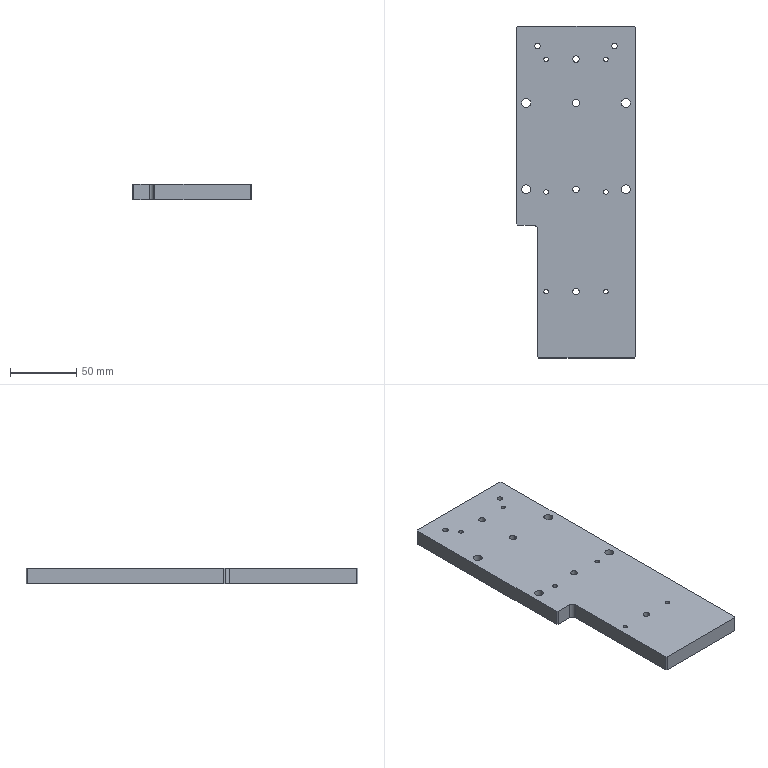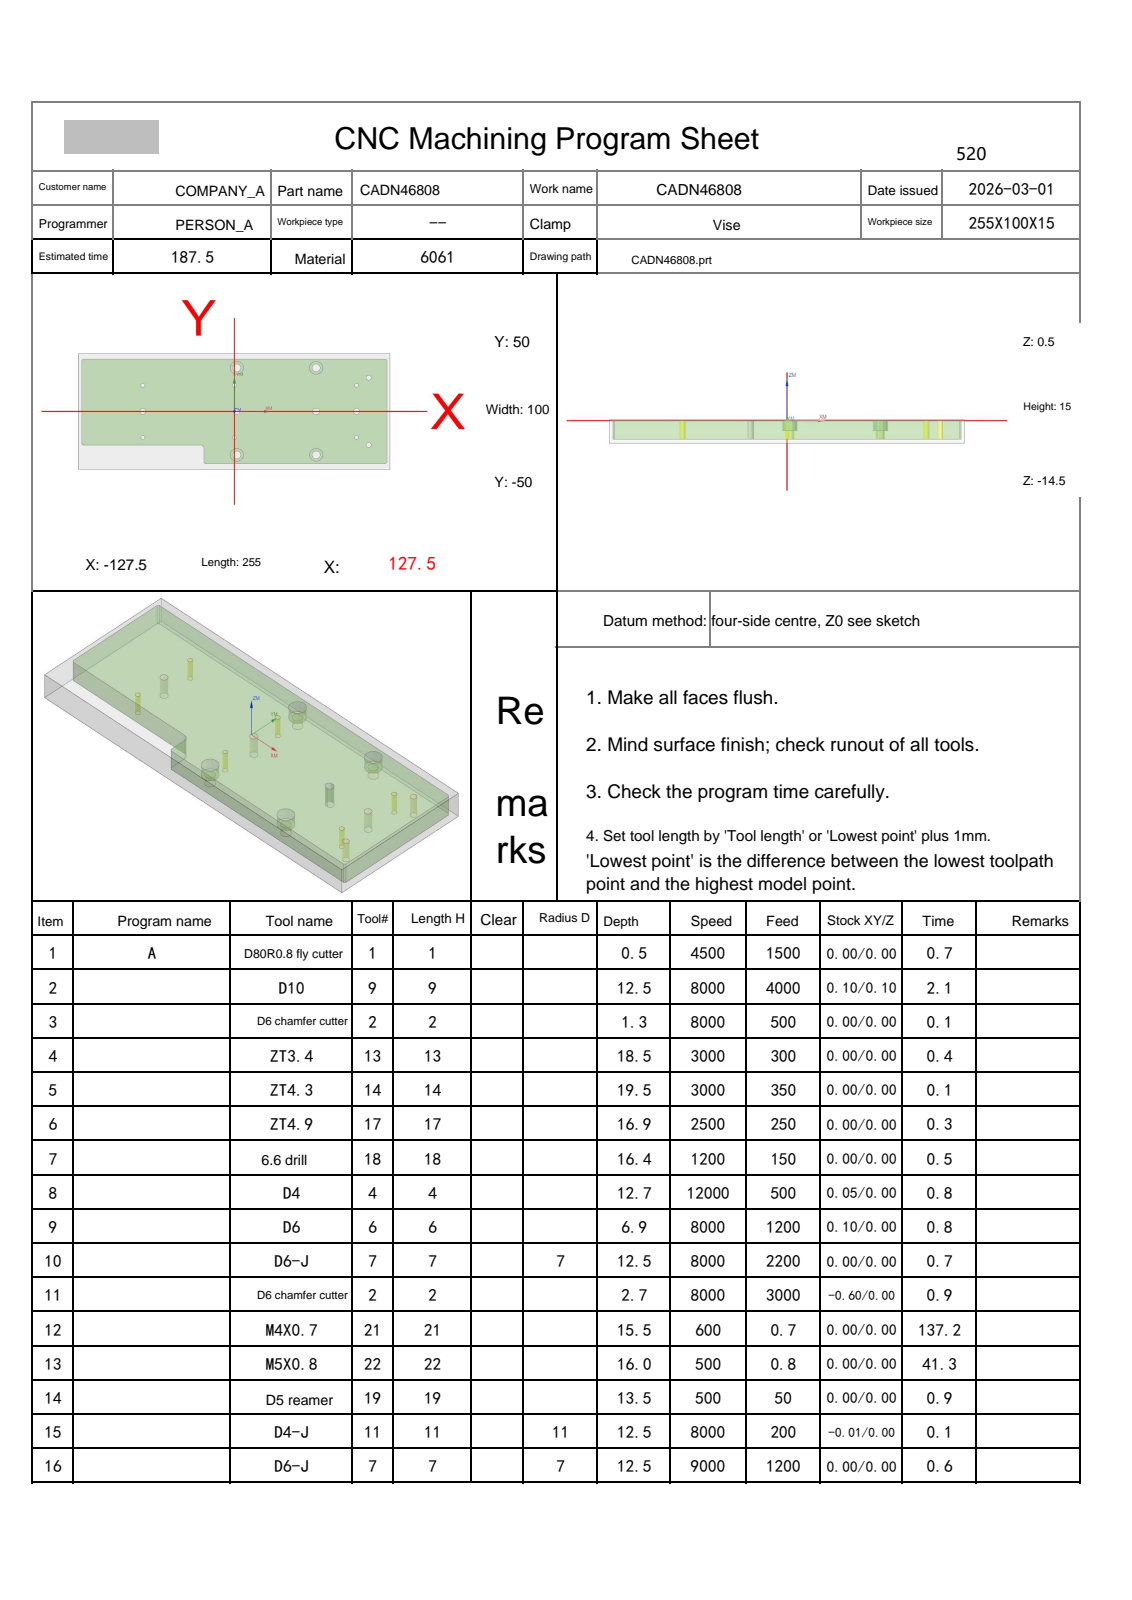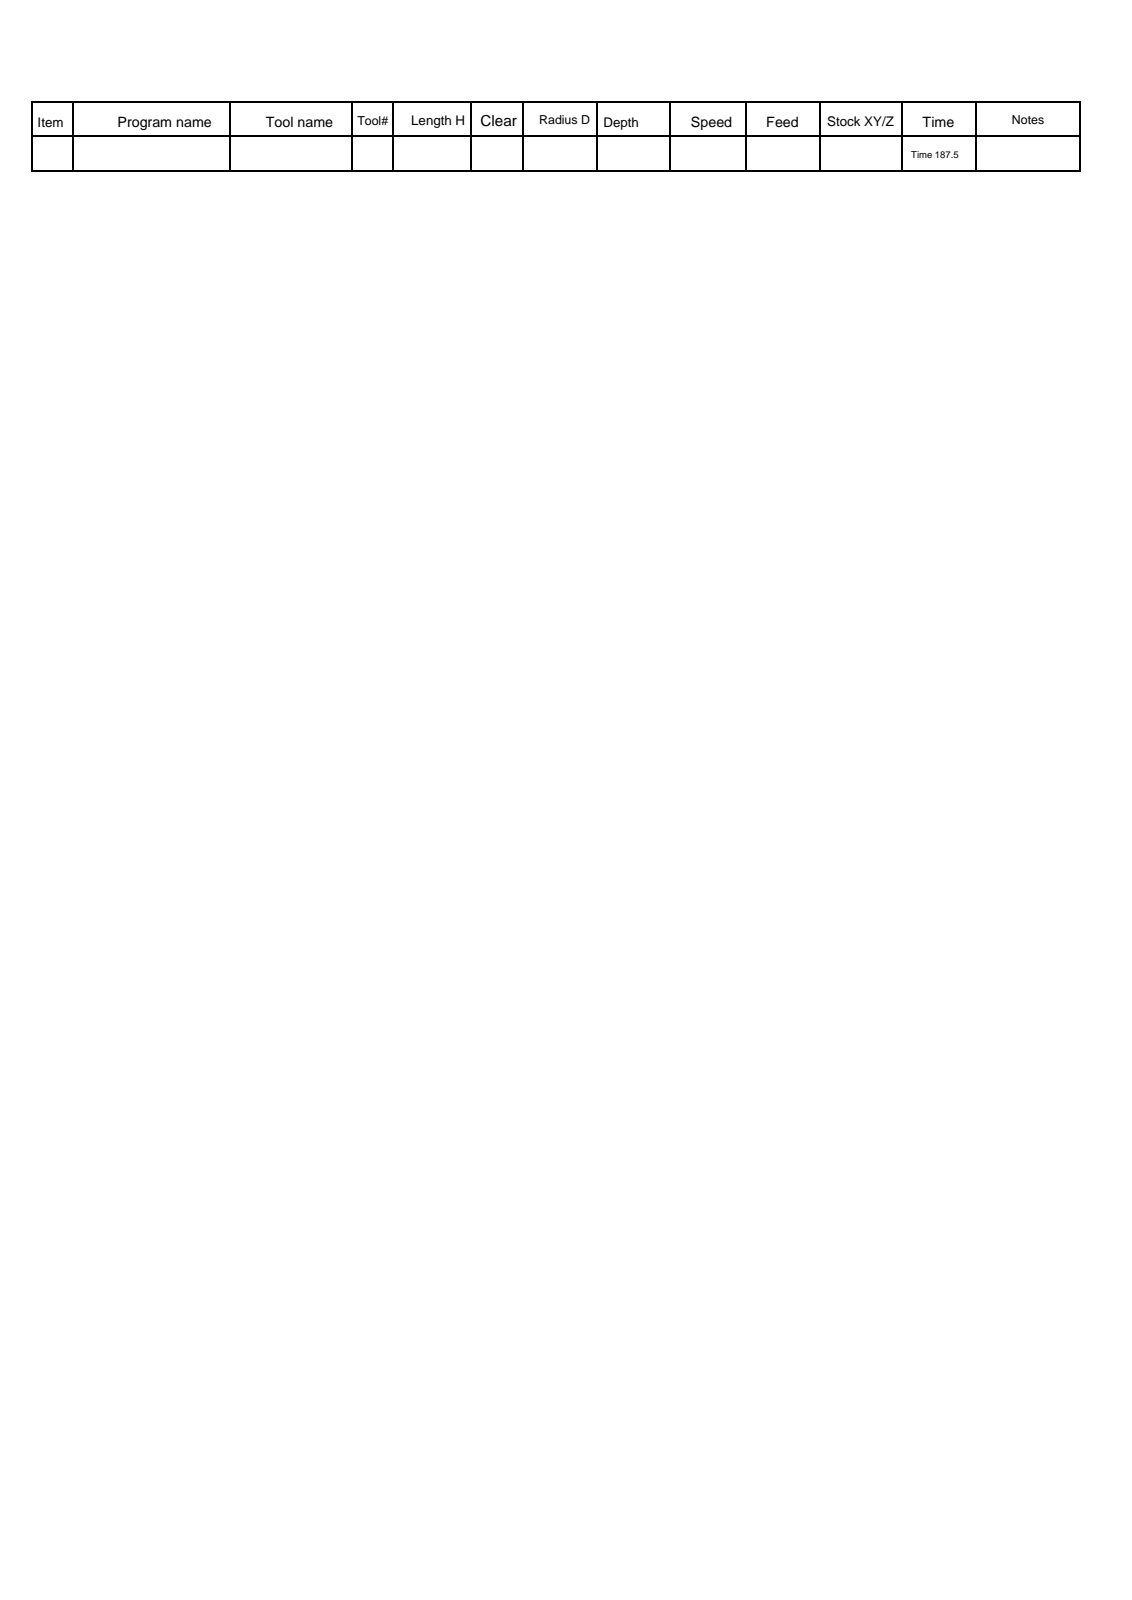NC program | NX | posted by the shop | part box 90 x 250 x 12 mm
Lines 1514 to 3445 of 3445, first 1356 of 1932 lines:
N10 T07 M06
(D6-J  D=6. R=0. H=07 ce=0.00 di=0.00)
G00 G90 G54 X2. Y-37.5 M03 S8000
G43 H07 Z50.
M08
Z0.0
G41 D07
G01 X2.197 Y-37.468 F500.
G03 X3.242 Y-36.242 I-.197 J1.226
X2. Y-35. I-1.242 J0.0
X2. Y-35. Z-5. I0.0 J-2.5
X-.456 Y-37.968 Z-6.4 I0.0 J-2.5
X2. Y-40. I2.456 J.468
X4.5 Y-37.5 I0.0 J2.5
X2. Y-35. I-2.5 J0.0
X-.5 Y-37.5 I0.0 J-2.5
X-.456 Y-37.968 I2.5 J0.0
X.764 Y-38.978 I1.22 J.233
X2.006 Y-37.736 I0.0 J1.242
G01 Y-37.7
G40 X2. Y-37.5
G00 Z50.
X67.
Z0.0
G41 D07
G01 X67.197 Y-37.468
G03 X68.242 Y-36.242 I-.197 J1.226
X67. Y-35. I-1.242 J0.0
X67. Y-35. Z-5. I0.0 J-2.5
X64.544 Y-37.968 Z-6.4 I0.0 J-2.5
X67. Y-40. I2.456 J.468
X69.5 Y-37.5 I0.0 J2.5
X67. Y-35. I-2.5 J0.0
X64.5 Y-37.5 I0.0 J-2.5
X64.544 Y-37.968 I2.5 J0.0
X65.764 Y-38.978 I1.22 J.233
X67.006 Y-37.736 I0.0 J1.242
G01 Y-37.7
G40 X67. Y-37.5
G00 Z50.
Y37.5
Z0.0
G41 D07
G01 X67.197 Y37.532
G03 X68.242 Y38.758 I-.197 J1.226
X67. Y40. I-1.242 J0.0
X67. Y40. Z-5. I0.0 J-2.5
X64.544 Y37.032 Z-6.4 I0.0 J-2.5
X67. Y35. I2.456 J.468
X69.5 Y37.5 I0.0 J2.5
X67. Y40. I-2.5 J0.0
X64.5 Y37.5 I0.0 J-2.5
X64.544 Y37.032 I2.5 J0.0
X65.764 Y36.022 I1.22 J.233
X67.006 Y37.264 I0.0 J1.242
G01 Y37.3
G40 X67. Y37.5
G00 Z50.
X2.
Z0.0
G41 D07
G01 X2.197 Y37.532
G03 X3.242 Y38.758 I-.197 J1.226
X2. Y40. I-1.242 J0.0
X2. Y40. Z-5. I0.0 J-2.5
X-.456 Y37.032 Z-6.4 I0.0 J-2.5
X2. Y35. I2.456 J.468
X4.5 Y37.5 I0.0 J2.5
X2. Y40. I-2.5 J0.0
X-.5 Y37.5 I0.0 J-2.5
X-.456 Y37.032 I2.5 J0.0
X.764 Y36.022 I1.22 J.233
X2.006 Y37.264 I0.0 J1.242
G01 Y37.3
G40 X2. Y37.5
G00 Z50.
G00 G90 X-28.61 Y-35.604 M03 S8000
Z50.
Z.35
G01 X-28.602 Y-35.602 Z.259 F2200.
X-28.581 Y-35.597 Z.177
X-28.547 Y-35.587 Z.103
X-28.503 Y-35.573 Z.038
X-28.452 Y-35.555 Z-.019
X-28.395 Y-35.531 Z-.069
X-28.336 Y-35.501 Z-.111
X-28.275 Y-35.465 Z-.147
X-28.215 Y-35.422 Z-.177
X-28.158 Y-35.372 Z-.201
X-28.107 Y-35.315 Z-.22
X-28.063 Y-35.25 Z-.234
X-28.03 Y-35.176 Z-.243
X-28.008 Y-35.094 Z-.248
X-28. Y-35.003 Z-.25
Y-32.
X-31.003
X-31.072 Y-32.016 Z-.251
X-31.117 Y-32.062 Z-.253
X-31.139 Y-32.135 Z-.256
X-31.141 Y-32.231 Z-.261
X-31.124 Y-32.347 Z-.267
X-31.089 Y-32.479 Z-.274
X-31.039 Y-32.624 Z-.281
X-30.975 Y-32.778 Z-.29
X-30.899 Y-32.939 Z-.298
X-30.812 Y-33.102 Z-.308
X-30.717 Y-33.264 Z-.318
X-30.484 Y-33.605 Z-.34
X-30.221 Y-33.924 Z-.363
X-29.929 Y-34.217 Z-.387
X-29.61 Y-34.481 Z-.41
X-29.268 Y-34.715 Z-.432
X-29.106 Y-34.81 Z-.442
X-28.943 Y-34.897 Z-.452
X-28.782 Y-34.973 Z-.46
X-28.627 Y-35.038 Z-.469
X-28.481 Y-35.088 Z-.476
X-28.349 Y-35.123 Z-.483
X-28.232 Y-35.141 Z-.489
X-28.136 Y-35.139 Z-.494
X-28.063 Y-35.117 Z-.497
X-28.016 Y-35.072 Z-.499
X-28. Y-35.003 Z-.5
Y-32.
X-31.003
X-31.072 Y-32.016 Z-.501
X-31.117 Y-32.062 Z-.503
X-31.139 Y-32.135 Z-.506
X-31.141 Y-32.231 Z-.511
X-31.124 Y-32.347 Z-.517
X-31.089 Y-32.479 Z-.524
X-31.039 Y-32.624 Z-.531
X-30.975 Y-32.778 Z-.54
X-30.899 Y-32.939 Z-.548
X-30.812 Y-33.102 Z-.558
X-30.717 Y-33.264 Z-.568
X-30.484 Y-33.605 Z-.59
X-30.221 Y-33.924 Z-.613
X-29.929 Y-34.217 Z-.637
X-29.61 Y-34.481 Z-.66
X-29.268 Y-34.715 Z-.682
X-29.106 Y-34.81 Z-.692
X-28.943 Y-34.897 Z-.702
X-28.782 Y-34.973 Z-.71
X-28.627 Y-35.038 Z-.719
X-28.481 Y-35.088 Z-.726
X-28.349 Y-35.123 Z-.733
X-28.232 Y-35.141 Z-.739
X-28.136 Y-35.139 Z-.744
X-28.063 Y-35.117 Z-.747
X-28.016 Y-35.072 Z-.749
X-28. Y-35.003 Z-.75
Y-32.
X-31.003
X-31.072 Y-32.016 Z-.751
X-31.117 Y-32.062 Z-.753
X-31.139 Y-32.135 Z-.756
X-31.141 Y-32.231 Z-.761
X-31.124 Y-32.347 Z-.767
X-31.089 Y-32.479 Z-.774
X-31.039 Y-32.624 Z-.781
X-30.975 Y-32.778 Z-.79
X-30.899 Y-32.939 Z-.798
X-30.812 Y-33.102 Z-.808
X-30.717 Y-33.264 Z-.818
X-30.484 Y-33.605 Z-.84
X-30.221 Y-33.924 Z-.863
X-29.929 Y-34.217 Z-.887
X-29.61 Y-34.481 Z-.91
X-29.268 Y-34.715 Z-.932
X-29.106 Y-34.81 Z-.942
X-28.943 Y-34.897 Z-.952
X-28.782 Y-34.973 Z-.96
X-28.627 Y-35.038 Z-.969
X-28.481 Y-35.088 Z-.976
X-28.349 Y-35.123 Z-.983
X-28.232 Y-35.141 Z-.989
X-28.136 Y-35.139 Z-.994
X-28.063 Y-35.117 Z-.997
X-28.016 Y-35.072 Z-.999
X-28. Y-35.003 Z-1.
Y-32.
X-31.003
X-31.072 Y-32.016 Z-1.001
X-31.117 Y-32.062 Z-1.003
X-31.139 Y-32.135 Z-1.006
X-31.141 Y-32.231 Z-1.011
X-31.124 Y-32.347 Z-1.017
X-31.089 Y-32.479 Z-1.024
X-31.039 Y-32.624 Z-1.031
X-30.975 Y-32.778 Z-1.04
X-30.899 Y-32.939 Z-1.048
X-30.812 Y-33.102 Z-1.058
X-30.717 Y-33.264 Z-1.068
X-30.484 Y-33.605 Z-1.09
X-30.221 Y-33.924 Z-1.113
X-29.929 Y-34.217 Z-1.137
X-29.61 Y-34.481 Z-1.16
X-29.268 Y-34.715 Z-1.182
X-29.106 Y-34.81 Z-1.192
X-28.943 Y-34.897 Z-1.202
X-28.782 Y-34.973 Z-1.21
X-28.627 Y-35.038 Z-1.219
X-28.481 Y-35.088 Z-1.226
X-28.349 Y-35.123 Z-1.233
X-28.232 Y-35.141 Z-1.239
X-28.136 Y-35.139 Z-1.244
X-28.063 Y-35.117 Z-1.247
X-28.016 Y-35.072 Z-1.249
X-28. Y-35.003 Z-1.25
Y-32.
X-31.003
X-31.072 Y-32.016 Z-1.251
X-31.117 Y-32.062 Z-1.253
X-31.139 Y-32.135 Z-1.256
X-31.141 Y-32.231 Z-1.261
X-31.124 Y-32.347 Z-1.267
X-31.089 Y-32.479 Z-1.274
X-31.039 Y-32.624 Z-1.281
X-30.975 Y-32.778 Z-1.29
X-30.899 Y-32.939 Z-1.298
X-30.812 Y-33.102 Z-1.308
X-30.717 Y-33.264 Z-1.318
X-30.484 Y-33.605 Z-1.34
X-30.221 Y-33.924 Z-1.363
X-29.929 Y-34.217 Z-1.387
X-29.61 Y-34.481 Z-1.41
X-29.268 Y-34.715 Z-1.432
X-29.106 Y-34.81 Z-1.442
X-28.943 Y-34.897 Z-1.452
X-28.782 Y-34.973 Z-1.46
X-28.627 Y-35.038 Z-1.469
X-28.481 Y-35.088 Z-1.476
X-28.349 Y-35.123 Z-1.483
X-28.232 Y-35.141 Z-1.489
X-28.136 Y-35.139 Z-1.494
X-28.063 Y-35.117 Z-1.497
X-28.016 Y-35.072 Z-1.499
X-28. Y-35.003 Z-1.5
Y-32.
X-31.003
X-31.072 Y-32.016 Z-1.501
X-31.117 Y-32.062 Z-1.503
X-31.139 Y-32.135 Z-1.506
X-31.141 Y-32.231 Z-1.511
X-31.124 Y-32.347 Z-1.517
X-31.089 Y-32.479 Z-1.524
X-31.039 Y-32.624 Z-1.531
X-30.975 Y-32.778 Z-1.54
X-30.899 Y-32.939 Z-1.548
X-30.812 Y-33.102 Z-1.558
X-30.717 Y-33.264 Z-1.568
X-30.484 Y-33.605 Z-1.59
X-30.221 Y-33.924 Z-1.613
X-29.929 Y-34.217 Z-1.637
X-29.61 Y-34.481 Z-1.66
X-29.268 Y-34.715 Z-1.682
X-29.106 Y-34.81 Z-1.692
X-28.943 Y-34.897 Z-1.702
X-28.782 Y-34.973 Z-1.71
X-28.627 Y-35.038 Z-1.719
X-28.481 Y-35.088 Z-1.726
X-28.349 Y-35.123 Z-1.733
X-28.232 Y-35.141 Z-1.739
X-28.136 Y-35.139 Z-1.744
X-28.063 Y-35.117 Z-1.747
X-28.016 Y-35.072 Z-1.749
X-28. Y-35.003 Z-1.75
Y-32.
X-31.003
X-31.072 Y-32.016 Z-1.751
X-31.117 Y-32.062 Z-1.753
X-31.139 Y-32.135 Z-1.756
X-31.141 Y-32.231 Z-1.761
X-31.124 Y-32.347 Z-1.767
X-31.089 Y-32.479 Z-1.774
X-31.039 Y-32.624 Z-1.781
X-30.975 Y-32.778 Z-1.79
X-30.899 Y-32.939 Z-1.798
X-30.812 Y-33.102 Z-1.808
X-30.717 Y-33.264 Z-1.818
X-30.484 Y-33.605 Z-1.84
X-30.221 Y-33.924 Z-1.863
X-29.929 Y-34.217 Z-1.887
X-29.61 Y-34.481 Z-1.91
X-29.268 Y-34.715 Z-1.932
X-29.106 Y-34.81 Z-1.942
X-28.943 Y-34.897 Z-1.952
X-28.782 Y-34.973 Z-1.96
X-28.627 Y-35.038 Z-1.969
X-28.481 Y-35.088 Z-1.976
X-28.349 Y-35.123 Z-1.983
X-28.232 Y-35.141 Z-1.989
X-28.136 Y-35.139 Z-1.994
X-28.063 Y-35.117 Z-1.997
X-28.016 Y-35.072 Z-1.999
X-28. Y-35.003 Z-2.
Y-32.
X-31.003
X-31.072 Y-32.016 Z-2.001
X-31.117 Y-32.062 Z-2.003
X-31.139 Y-32.135 Z-2.006
X-31.141 Y-32.231 Z-2.011
X-31.124 Y-32.347 Z-2.017
X-31.089 Y-32.479 Z-2.024
X-31.039 Y-32.624 Z-2.031
X-30.975 Y-32.778 Z-2.04
X-30.899 Y-32.939 Z-2.048
X-30.812 Y-33.102 Z-2.058
X-30.717 Y-33.264 Z-2.068
X-30.484 Y-33.605 Z-2.09
X-30.221 Y-33.924 Z-2.113
X-29.929 Y-34.217 Z-2.137
X-29.61 Y-34.481 Z-2.16
X-29.268 Y-34.715 Z-2.182
X-29.106 Y-34.81 Z-2.192
X-28.943 Y-34.897 Z-2.202
X-28.782 Y-34.973 Z-2.21
X-28.627 Y-35.038 Z-2.219
X-28.481 Y-35.088 Z-2.226
X-28.349 Y-35.123 Z-2.233
X-28.232 Y-35.141 Z-2.239
X-28.136 Y-35.139 Z-2.244
X-28.063 Y-35.117 Z-2.247
X-28.016 Y-35.072 Z-2.249
X-28. Y-35.003 Z-2.25
Y-32.
X-31.003
X-31.072 Y-32.016 Z-2.251
X-31.117 Y-32.062 Z-2.253
X-31.139 Y-32.135 Z-2.256
X-31.141 Y-32.231 Z-2.261
X-31.124 Y-32.347 Z-2.267
X-31.089 Y-32.479 Z-2.274
X-31.039 Y-32.624 Z-2.281
X-30.975 Y-32.778 Z-2.29
X-30.899 Y-32.939 Z-2.298
X-30.812 Y-33.102 Z-2.308
X-30.717 Y-33.264 Z-2.318
X-30.484 Y-33.605 Z-2.34
X-30.221 Y-33.924 Z-2.363
X-29.929 Y-34.217 Z-2.387
X-29.61 Y-34.481 Z-2.41
X-29.268 Y-34.715 Z-2.432
X-29.106 Y-34.81 Z-2.442
X-28.943 Y-34.897 Z-2.452
X-28.782 Y-34.973 Z-2.46
X-28.627 Y-35.038 Z-2.469
X-28.481 Y-35.088 Z-2.476
X-28.349 Y-35.123 Z-2.483
X-28.232 Y-35.141 Z-2.489
X-28.136 Y-35.139 Z-2.494
X-28.063 Y-35.117 Z-2.497
X-28.016 Y-35.072 Z-2.499
X-28. Y-35.003 Z-2.5
Y-32.
X-31.003
X-31.072 Y-32.016 Z-2.501
X-31.117 Y-32.062 Z-2.503
X-31.139 Y-32.135 Z-2.506
X-31.141 Y-32.231 Z-2.511
X-31.124 Y-32.347 Z-2.517
X-31.089 Y-32.479 Z-2.524
X-31.039 Y-32.624 Z-2.531
X-30.975 Y-32.778 Z-2.54
X-30.899 Y-32.939 Z-2.548
X-30.812 Y-33.102 Z-2.558
X-30.717 Y-33.264 Z-2.568
X-30.484 Y-33.605 Z-2.59
X-30.221 Y-33.924 Z-2.613
X-29.929 Y-34.217 Z-2.637
X-29.61 Y-34.481 Z-2.66
X-29.268 Y-34.715 Z-2.682
X-29.106 Y-34.81 Z-2.692
X-28.943 Y-34.897 Z-2.702
X-28.782 Y-34.973 Z-2.71
X-28.627 Y-35.038 Z-2.719
X-28.481 Y-35.088 Z-2.726
X-28.349 Y-35.123 Z-2.733
X-28.232 Y-35.141 Z-2.739
X-28.136 Y-35.139 Z-2.744
X-28.063 Y-35.117 Z-2.747
X-28.016 Y-35.072 Z-2.749
X-28. Y-35.003 Z-2.75
Y-32.
X-31.003
X-31.072 Y-32.016 Z-2.751
X-31.117 Y-32.062 Z-2.753
X-31.139 Y-32.135 Z-2.756
X-31.141 Y-32.231 Z-2.761
X-31.124 Y-32.347 Z-2.767
X-31.089 Y-32.479 Z-2.774
X-31.039 Y-32.624 Z-2.781
X-30.975 Y-32.778 Z-2.79
X-30.899 Y-32.939 Z-2.798
X-30.812 Y-33.102 Z-2.808
X-30.717 Y-33.264 Z-2.818
X-30.484 Y-33.605 Z-2.84
X-30.221 Y-33.924 Z-2.863
X-29.929 Y-34.217 Z-2.887
X-29.61 Y-34.481 Z-2.91
X-29.268 Y-34.715 Z-2.932
X-29.106 Y-34.81 Z-2.942
X-28.943 Y-34.897 Z-2.952
X-28.782 Y-34.973 Z-2.96
X-28.627 Y-35.038 Z-2.969
X-28.481 Y-35.088 Z-2.976
X-28.349 Y-35.123 Z-2.983
X-28.232 Y-35.141 Z-2.989
X-28.136 Y-35.139 Z-2.994
X-28.063 Y-35.117 Z-2.997
X-28.016 Y-35.072 Z-2.999
X-28. Y-35.003 Z-3.
Y-32.
X-31.003
X-31.072 Y-32.016 Z-3.001
X-31.117 Y-32.062 Z-3.003
X-31.139 Y-32.135 Z-3.006
X-31.141 Y-32.231 Z-3.011
X-31.124 Y-32.347 Z-3.017
X-31.089 Y-32.479 Z-3.024
X-31.039 Y-32.624 Z-3.031
X-30.975 Y-32.778 Z-3.04
X-30.899 Y-32.939 Z-3.048
X-30.812 Y-33.102 Z-3.058
X-30.717 Y-33.264 Z-3.068
X-30.484 Y-33.605 Z-3.09
X-30.221 Y-33.924 Z-3.113
X-29.929 Y-34.217 Z-3.137
X-29.61 Y-34.481 Z-3.16
X-29.268 Y-34.715 Z-3.182
X-29.106 Y-34.81 Z-3.192
X-28.943 Y-34.897 Z-3.202
X-28.782 Y-34.973 Z-3.21
X-28.627 Y-35.038 Z-3.219
X-28.481 Y-35.088 Z-3.226
X-28.349 Y-35.123 Z-3.233
X-28.232 Y-35.141 Z-3.239
X-28.136 Y-35.139 Z-3.244
X-28.063 Y-35.117 Z-3.247
X-28.016 Y-35.072 Z-3.249
X-28. Y-35.003 Z-3.25
Y-32.
X-31.003
X-31.072 Y-32.016 Z-3.251
X-31.117 Y-32.062 Z-3.253
X-31.139 Y-32.135 Z-3.256
X-31.141 Y-32.231 Z-3.261
X-31.124 Y-32.347 Z-3.267
X-31.089 Y-32.479 Z-3.274
X-31.039 Y-32.624 Z-3.281
X-30.975 Y-32.778 Z-3.29
X-30.899 Y-32.939 Z-3.298
X-30.812 Y-33.102 Z-3.308
X-30.717 Y-33.264 Z-3.318
X-30.484 Y-33.605 Z-3.34
X-30.221 Y-33.924 Z-3.363
X-29.929 Y-34.217 Z-3.387
X-29.61 Y-34.481 Z-3.41
X-29.268 Y-34.715 Z-3.432
X-29.106 Y-34.81 Z-3.442
X-28.943 Y-34.897 Z-3.452
X-28.782 Y-34.973 Z-3.46
X-28.627 Y-35.038 Z-3.469
X-28.481 Y-35.088 Z-3.476
X-28.349 Y-35.123 Z-3.483
X-28.232 Y-35.141 Z-3.489
X-28.136 Y-35.139 Z-3.494
X-28.063 Y-35.117 Z-3.497
X-28.016 Y-35.072 Z-3.499
X-28. Y-35.003 Z-3.5
Y-32.
X-31.003
X-31.072 Y-32.016 Z-3.501
X-31.117 Y-32.062 Z-3.503
X-31.139 Y-32.135 Z-3.506
X-31.141 Y-32.231 Z-3.511
X-31.124 Y-32.347 Z-3.517
X-31.089 Y-32.479 Z-3.524
X-31.039 Y-32.624 Z-3.531
X-30.975 Y-32.778 Z-3.54
X-30.899 Y-32.939 Z-3.548
X-30.812 Y-33.102 Z-3.558
X-30.717 Y-33.264 Z-3.568
X-30.484 Y-33.605 Z-3.59
X-30.221 Y-33.924 Z-3.613
X-29.929 Y-34.217 Z-3.637
X-29.61 Y-34.481 Z-3.66
X-29.268 Y-34.715 Z-3.682
X-29.106 Y-34.81 Z-3.692
X-28.943 Y-34.897 Z-3.702
X-28.782 Y-34.973 Z-3.71
X-28.627 Y-35.038 Z-3.719
X-28.481 Y-35.088 Z-3.726
X-28.349 Y-35.123 Z-3.733
X-28.232 Y-35.141 Z-3.739
X-28.136 Y-35.139 Z-3.744
X-28.063 Y-35.117 Z-3.747
X-28.016 Y-35.072 Z-3.749
X-28. Y-35.003 Z-3.75
Y-32.
X-31.003
X-31.072 Y-32.016 Z-3.751
X-31.117 Y-32.062 Z-3.753
X-31.139 Y-32.135 Z-3.756
X-31.141 Y-32.231 Z-3.761
X-31.124 Y-32.347 Z-3.767
X-31.089 Y-32.479 Z-3.774
X-31.039 Y-32.624 Z-3.781
X-30.975 Y-32.778 Z-3.79
X-30.899 Y-32.939 Z-3.798
X-30.812 Y-33.102 Z-3.808
X-30.717 Y-33.264 Z-3.818
X-30.484 Y-33.605 Z-3.84
X-30.221 Y-33.924 Z-3.863
X-29.929 Y-34.217 Z-3.887
X-29.61 Y-34.481 Z-3.91
X-29.268 Y-34.715 Z-3.932
X-29.106 Y-34.81 Z-3.942
X-28.943 Y-34.897 Z-3.952
X-28.782 Y-34.973 Z-3.96
X-28.627 Y-35.038 Z-3.969
X-28.481 Y-35.088 Z-3.976
X-28.349 Y-35.123 Z-3.983
X-28.232 Y-35.141 Z-3.989
X-28.136 Y-35.139 Z-3.994
X-28.063 Y-35.117 Z-3.997
X-28.016 Y-35.072 Z-3.999
X-28. Y-35.003 Z-4.
Y-32.
X-31.003
X-31.072 Y-32.016 Z-4.001
X-31.117 Y-32.062 Z-4.003
X-31.139 Y-32.135 Z-4.006
X-31.141 Y-32.231 Z-4.011
X-31.124 Y-32.347 Z-4.017
X-31.089 Y-32.479 Z-4.024
X-31.039 Y-32.624 Z-4.031
X-30.975 Y-32.778 Z-4.04
X-30.899 Y-32.939 Z-4.048
X-30.812 Y-33.102 Z-4.058
X-30.717 Y-33.264 Z-4.068
X-30.484 Y-33.605 Z-4.09
X-30.221 Y-33.924 Z-4.113
X-29.929 Y-34.217 Z-4.137
X-29.61 Y-34.481 Z-4.16
X-29.268 Y-34.715 Z-4.182
X-29.106 Y-34.81 Z-4.192
X-28.943 Y-34.897 Z-4.202
X-28.782 Y-34.973 Z-4.21
X-28.627 Y-35.038 Z-4.219
X-28.481 Y-35.088 Z-4.226
X-28.349 Y-35.123 Z-4.233
X-28.232 Y-35.141 Z-4.239
X-28.136 Y-35.139 Z-4.244
X-28.063 Y-35.117 Z-4.247
X-28.016 Y-35.072 Z-4.249
X-28. Y-35.003 Z-4.25
Y-32.
X-31.003
X-31.072 Y-32.016 Z-4.251
X-31.117 Y-32.062 Z-4.253
X-31.139 Y-32.135 Z-4.256
X-31.141 Y-32.231 Z-4.261
X-31.124 Y-32.347 Z-4.267
X-31.089 Y-32.479 Z-4.274
X-31.039 Y-32.624 Z-4.281
X-30.975 Y-32.778 Z-4.29
X-30.899 Y-32.939 Z-4.298
X-30.812 Y-33.102 Z-4.308
X-30.717 Y-33.264 Z-4.318
X-30.484 Y-33.605 Z-4.34
X-30.221 Y-33.924 Z-4.363
X-29.929 Y-34.217 Z-4.387
X-29.61 Y-34.481 Z-4.41
X-29.268 Y-34.715 Z-4.432
X-29.106 Y-34.81 Z-4.442
X-28.943 Y-34.897 Z-4.452
X-28.782 Y-34.973 Z-4.46
X-28.627 Y-35.038 Z-4.469
X-28.481 Y-35.088 Z-4.476
X-28.349 Y-35.123 Z-4.483
X-28.232 Y-35.141 Z-4.489
X-28.136 Y-35.139 Z-4.494
X-28.063 Y-35.117 Z-4.497
X-28.016 Y-35.072 Z-4.499
X-28. Y-35.003 Z-4.5
Y-32.
X-31.003
X-31.072 Y-32.016 Z-4.501
X-31.117 Y-32.062 Z-4.503
X-31.139 Y-32.135 Z-4.506
X-31.141 Y-32.231 Z-4.511
X-31.124 Y-32.347 Z-4.517
X-31.089 Y-32.479 Z-4.524
X-31.039 Y-32.624 Z-4.531
X-30.975 Y-32.778 Z-4.54
X-30.899 Y-32.939 Z-4.548
X-30.812 Y-33.102 Z-4.558
X-30.717 Y-33.264 Z-4.568
X-30.484 Y-33.605 Z-4.59
X-30.221 Y-33.924 Z-4.613
X-29.929 Y-34.217 Z-4.637
X-29.61 Y-34.481 Z-4.66
X-29.268 Y-34.715 Z-4.682
X-29.106 Y-34.81 Z-4.692
X-28.943 Y-34.897 Z-4.702
X-28.782 Y-34.973 Z-4.71
X-28.627 Y-35.038 Z-4.719
X-28.481 Y-35.088 Z-4.726
X-28.349 Y-35.123 Z-4.733
X-28.232 Y-35.141 Z-4.739
X-28.136 Y-35.139 Z-4.744
X-28.063 Y-35.117 Z-4.747
X-28.016 Y-35.072 Z-4.749
X-28. Y-35.003 Z-4.75
Y-32.
X-31.003
X-31.072 Y-32.016 Z-4.751
X-31.117 Y-32.062 Z-4.753
X-31.139 Y-32.135 Z-4.756
X-31.141 Y-32.231 Z-4.761
X-31.124 Y-32.347 Z-4.767
X-31.089 Y-32.479 Z-4.774
X-31.039 Y-32.624 Z-4.781
X-30.975 Y-32.778 Z-4.79
X-30.899 Y-32.939 Z-4.798
X-30.812 Y-33.102 Z-4.808
X-30.717 Y-33.264 Z-4.818
X-30.484 Y-33.605 Z-4.84
X-30.221 Y-33.924 Z-4.863
X-29.929 Y-34.217 Z-4.887
X-29.61 Y-34.481 Z-4.91
X-29.268 Y-34.715 Z-4.932
X-29.106 Y-34.81 Z-4.942
X-28.943 Y-34.897 Z-4.952
X-28.782 Y-34.973 Z-4.96
X-28.627 Y-35.038 Z-4.969
X-28.481 Y-35.088 Z-4.976
X-28.349 Y-35.123 Z-4.983
X-28.232 Y-35.141 Z-4.989
X-28.136 Y-35.139 Z-4.994
X-28.063 Y-35.117 Z-4.997
X-28.016 Y-35.072 Z-4.999
X-28. Y-35.003 Z-5.
Y-32.
X-31.003
X-31.072 Y-32.016 Z-5.001
X-31.117 Y-32.062 Z-5.003
X-31.139 Y-32.135 Z-5.006
X-31.141 Y-32.231 Z-5.011
X-31.124 Y-32.347 Z-5.017
X-31.089 Y-32.479 Z-5.024
X-31.039 Y-32.624 Z-5.031
X-30.975 Y-32.778 Z-5.04
X-30.899 Y-32.939 Z-5.048
X-30.812 Y-33.102 Z-5.058
X-30.717 Y-33.264 Z-5.068
X-30.484 Y-33.605 Z-5.09
X-30.221 Y-33.924 Z-5.113
X-29.929 Y-34.217 Z-5.137
X-29.61 Y-34.481 Z-5.16
X-29.268 Y-34.715 Z-5.182
X-29.106 Y-34.81 Z-5.192
X-28.943 Y-34.897 Z-5.202
X-28.782 Y-34.973 Z-5.21
X-28.627 Y-35.038 Z-5.219
X-28.481 Y-35.088 Z-5.226
X-28.349 Y-35.123 Z-5.233
X-28.232 Y-35.141 Z-5.239
X-28.136 Y-35.139 Z-5.244
X-28.063 Y-35.117 Z-5.247
X-28.016 Y-35.072 Z-5.249
X-28. Y-35.003 Z-5.25
Y-32.
X-31.003
X-31.072 Y-32.016 Z-5.251
X-31.117 Y-32.062 Z-5.253
X-31.139 Y-32.135 Z-5.256
X-31.141 Y-32.231 Z-5.261
X-31.124 Y-32.347 Z-5.267
X-31.089 Y-32.479 Z-5.274
X-31.039 Y-32.624 Z-5.281
X-30.975 Y-32.778 Z-5.29
X-30.899 Y-32.939 Z-5.298
X-30.812 Y-33.102 Z-5.308
X-30.717 Y-33.264 Z-5.318
X-30.484 Y-33.605 Z-5.34
X-30.221 Y-33.924 Z-5.363
X-29.929 Y-34.217 Z-5.387
X-29.61 Y-34.481 Z-5.41
X-29.268 Y-34.715 Z-5.432
X-29.106 Y-34.81 Z-5.442
X-28.943 Y-34.897 Z-5.452
X-28.782 Y-34.973 Z-5.46
X-28.627 Y-35.038 Z-5.469
X-28.481 Y-35.088 Z-5.476
X-28.349 Y-35.123 Z-5.483
X-28.232 Y-35.141 Z-5.489
X-28.136 Y-35.139 Z-5.494
X-28.063 Y-35.117 Z-5.497
X-28.016 Y-35.072 Z-5.499
X-28. Y-35.003 Z-5.5
Y-32.
X-31.003
X-31.072 Y-32.016 Z-5.501
X-31.117 Y-32.062 Z-5.503
X-31.139 Y-32.135 Z-5.506
X-31.141 Y-32.231 Z-5.511
X-31.124 Y-32.347 Z-5.517
X-31.089 Y-32.479 Z-5.524
X-31.039 Y-32.624 Z-5.531
X-30.975 Y-32.778 Z-5.54
X-30.899 Y-32.939 Z-5.548
X-30.812 Y-33.102 Z-5.558
X-30.717 Y-33.264 Z-5.568
X-30.484 Y-33.605 Z-5.59
X-30.221 Y-33.924 Z-5.613
X-29.929 Y-34.217 Z-5.637
X-29.61 Y-34.481 Z-5.66
X-29.268 Y-34.715 Z-5.682
X-29.106 Y-34.81 Z-5.692
X-28.943 Y-34.897 Z-5.702
X-28.782 Y-34.973 Z-5.71
X-28.627 Y-35.038 Z-5.719
X-28.481 Y-35.088 Z-5.726
X-28.349 Y-35.123 Z-5.733
X-28.232 Y-35.141 Z-5.739
X-28.136 Y-35.139 Z-5.744
X-28.063 Y-35.117 Z-5.747
X-28.016 Y-35.072 Z-5.749
X-28. Y-35.003 Z-5.75
Y-32.
X-31.003
X-31.072 Y-32.016 Z-5.751
X-31.117 Y-32.062 Z-5.753
X-31.139 Y-32.135 Z-5.756
X-31.141 Y-32.231 Z-5.761
X-31.124 Y-32.347 Z-5.767
X-31.089 Y-32.479 Z-5.774
X-31.039 Y-32.624 Z-5.781
X-30.975 Y-32.778 Z-5.79
X-30.899 Y-32.939 Z-5.798
X-30.812 Y-33.102 Z-5.808
X-30.717 Y-33.264 Z-5.818
X-30.484 Y-33.605 Z-5.84
X-30.221 Y-33.924 Z-5.863
X-29.929 Y-34.217 Z-5.887
X-29.61 Y-34.481 Z-5.91
X-29.268 Y-34.715 Z-5.932
X-29.106 Y-34.81 Z-5.942
X-28.943 Y-34.897 Z-5.952
X-28.782 Y-34.973 Z-5.96
X-28.627 Y-35.038 Z-5.969
X-28.481 Y-35.088 Z-5.976
X-28.349 Y-35.123 Z-5.983
X-28.232 Y-35.141 Z-5.989
X-28.136 Y-35.139 Z-5.994
X-28.063 Y-35.117 Z-5.997
X-28.016 Y-35.072 Z-5.999
X-28. Y-35.003 Z-6.
Y-32.
X-31.003
X-31.072 Y-32.016 Z-6.001
X-31.117 Y-32.062 Z-6.003
X-31.139 Y-32.135 Z-6.006
X-31.141 Y-32.231 Z-6.011
X-31.124 Y-32.347 Z-6.017
X-31.089 Y-32.479 Z-6.024
X-31.039 Y-32.624 Z-6.031
X-30.975 Y-32.778 Z-6.04
X-30.899 Y-32.939 Z-6.048
X-30.812 Y-33.102 Z-6.058
X-30.717 Y-33.264 Z-6.068
X-30.484 Y-33.605 Z-6.09
X-30.221 Y-33.924 Z-6.113
X-29.929 Y-34.217 Z-6.137
X-29.61 Y-34.481 Z-6.16
X-29.268 Y-34.715 Z-6.182
X-29.106 Y-34.81 Z-6.192
X-28.943 Y-34.897 Z-6.202
X-28.782 Y-34.973 Z-6.21
X-28.627 Y-35.038 Z-6.219
X-28.481 Y-35.088 Z-6.226
X-28.349 Y-35.123 Z-6.233
X-28.232 Y-35.141 Z-6.239
X-28.136 Y-35.139 Z-6.244
X-28.063 Y-35.117 Z-6.247
X-28.016 Y-35.072 Z-6.249
X-28. Y-35.003 Z-6.25
Y-32.
X-31.003
X-31.072 Y-32.016 Z-6.251
X-31.117 Y-32.062 Z-6.253
X-31.139 Y-32.135 Z-6.256
X-31.141 Y-32.231 Z-6.261
X-31.124 Y-32.347 Z-6.267
X-31.089 Y-32.479 Z-6.274
X-31.039 Y-32.624 Z-6.281
X-30.975 Y-32.778 Z-6.29
X-30.899 Y-32.939 Z-6.298
X-30.812 Y-33.102 Z-6.308
X-30.717 Y-33.264 Z-6.318
X-30.484 Y-33.605 Z-6.34
X-30.221 Y-33.924 Z-6.363
X-29.929 Y-34.217 Z-6.387
X-29.61 Y-34.481 Z-6.41
X-29.268 Y-34.715 Z-6.432
X-29.106 Y-34.81 Z-6.442
X-28.943 Y-34.897 Z-6.452
X-28.782 Y-34.973 Z-6.46
X-28.627 Y-35.038 Z-6.469
X-28.481 Y-35.088 Z-6.476
X-28.349 Y-35.123 Z-6.483
X-28.232 Y-35.141 Z-6.489
X-28.136 Y-35.139 Z-6.494
X-28.063 Y-35.117 Z-6.497
X-28.016 Y-35.072 Z-6.499
X-28. Y-35.003 Z-6.5
Y-32.
X-31.003
X-31.072 Y-32.016 Z-6.501
X-31.117 Y-32.062 Z-6.503
X-31.139 Y-32.135 Z-6.506
X-31.141 Y-32.231 Z-6.511
X-31.124 Y-32.347 Z-6.517
X-31.089 Y-32.479 Z-6.524
X-31.039 Y-32.624 Z-6.531
X-30.975 Y-32.778 Z-6.54
X-30.899 Y-32.939 Z-6.548
X-30.812 Y-33.102 Z-6.558
X-30.717 Y-33.264 Z-6.568
X-30.484 Y-33.605 Z-6.59
X-30.221 Y-33.924 Z-6.613
X-29.929 Y-34.217 Z-6.637
X-29.61 Y-34.481 Z-6.66
X-29.268 Y-34.715 Z-6.682
X-29.106 Y-34.81 Z-6.692
X-28.943 Y-34.897 Z-6.702
X-28.782 Y-34.973 Z-6.71
X-28.627 Y-35.038 Z-6.719
X-28.481 Y-35.088 Z-6.726
X-28.349 Y-35.123 Z-6.733
X-28.232 Y-35.141 Z-6.739
X-28.136 Y-35.139 Z-6.744
X-28.063 Y-35.117 Z-6.747
X-28.016 Y-35.072 Z-6.749
X-28. Y-35.003 Z-6.75
Y-32.
X-31.003
X-31.072 Y-32.016 Z-6.751
X-31.117 Y-32.062 Z-6.753
X-31.139 Y-32.135 Z-6.756
X-31.141 Y-32.231 Z-6.761
X-31.124 Y-32.347 Z-6.767
X-31.089 Y-32.479 Z-6.774
X-31.039 Y-32.624 Z-6.781
X-30.975 Y-32.778 Z-6.79
X-30.899 Y-32.939 Z-6.798
X-30.812 Y-33.102 Z-6.808
X-30.717 Y-33.264 Z-6.818
X-30.484 Y-33.605 Z-6.84
X-30.221 Y-33.924 Z-6.863
X-29.929 Y-34.217 Z-6.887
X-29.61 Y-34.481 Z-6.91
X-29.268 Y-34.715 Z-6.932
X-29.106 Y-34.81 Z-6.942
X-28.943 Y-34.897 Z-6.952
X-28.782 Y-34.973 Z-6.96
X-28.627 Y-35.038 Z-6.969
X-28.481 Y-35.088 Z-6.976
X-28.349 Y-35.123 Z-6.983
X-28.232 Y-35.141 Z-6.989
X-28.136 Y-35.139 Z-6.994
X-28.063 Y-35.117 Z-6.997
X-28.016 Y-35.072 Z-6.999
X-28. Y-35.003 Z-7.
Y-32.
X-31.003
X-31.072 Y-32.016 Z-7.001
X-31.117 Y-32.062 Z-7.003
X-31.139 Y-32.135 Z-7.006
X-31.141 Y-32.231 Z-7.011
X-31.124 Y-32.347 Z-7.017
X-31.089 Y-32.479 Z-7.024
X-31.039 Y-32.624 Z-7.031
X-30.975 Y-32.778 Z-7.04
X-30.899 Y-32.939 Z-7.048
X-30.812 Y-33.102 Z-7.058
X-30.717 Y-33.264 Z-7.068
X-30.484 Y-33.605 Z-7.09
X-30.221 Y-33.924 Z-7.113
X-29.929 Y-34.217 Z-7.137
X-29.61 Y-34.481 Z-7.16
X-29.268 Y-34.715 Z-7.182
X-29.106 Y-34.81 Z-7.192
X-28.943 Y-34.897 Z-7.202
X-28.782 Y-34.973 Z-7.21
X-28.627 Y-35.038 Z-7.219
X-28.481 Y-35.088 Z-7.226
X-28.349 Y-35.123 Z-7.233
X-28.232 Y-35.141 Z-7.239
X-28.136 Y-35.139 Z-7.244
X-28.063 Y-35.117 Z-7.247
X-28.016 Y-35.072 Z-7.249
X-28. Y-35.003 Z-7.25
Y-32.
X-31.003
X-31.072 Y-32.016 Z-7.251
X-31.117 Y-32.062 Z-7.253
X-31.139 Y-32.135 Z-7.256
X-31.141 Y-32.231 Z-7.261
X-31.124 Y-32.347 Z-7.267
X-31.089 Y-32.479 Z-7.274
X-31.039 Y-32.624 Z-7.281
X-30.975 Y-32.778 Z-7.29
X-30.899 Y-32.939 Z-7.298
X-30.812 Y-33.102 Z-7.308
X-30.717 Y-33.264 Z-7.318
X-30.484 Y-33.605 Z-7.34
X-30.221 Y-33.924 Z-7.363
X-29.929 Y-34.217 Z-7.387
X-29.61 Y-34.481 Z-7.41
X-29.268 Y-34.715 Z-7.432
X-29.106 Y-34.81 Z-7.442
X-28.943 Y-34.897 Z-7.452
X-28.782 Y-34.973 Z-7.46
X-28.627 Y-35.038 Z-7.469
X-28.481 Y-35.088 Z-7.476
X-28.349 Y-35.123 Z-7.483
X-28.232 Y-35.141 Z-7.489
X-28.136 Y-35.139 Z-7.494
X-28.063 Y-35.117 Z-7.497
X-28.016 Y-35.072 Z-7.499
X-28. Y-35.003 Z-7.5
Y-32.
X-31.003
X-31.072 Y-32.016 Z-7.501
X-31.117 Y-32.062 Z-7.503
X-31.139 Y-32.135 Z-7.506
X-31.141 Y-32.231 Z-7.511
X-31.124 Y-32.347 Z-7.517
X-31.089 Y-32.479 Z-7.524
X-31.039 Y-32.624 Z-7.531
X-30.975 Y-32.778 Z-7.54
X-30.899 Y-32.939 Z-7.548
X-30.812 Y-33.102 Z-7.558
X-30.717 Y-33.264 Z-7.568
X-30.484 Y-33.605 Z-7.59
X-30.221 Y-33.924 Z-7.613
X-29.929 Y-34.217 Z-7.637
X-29.61 Y-34.481 Z-7.66
X-29.268 Y-34.715 Z-7.682
X-29.106 Y-34.81 Z-7.692
X-28.943 Y-34.897 Z-7.702
X-28.782 Y-34.973 Z-7.71
X-28.627 Y-35.038 Z-7.719
X-28.481 Y-35.088 Z-7.726
X-28.349 Y-35.123 Z-7.733
X-28.232 Y-35.141 Z-7.739
X-28.136 Y-35.139 Z-7.744
X-28.063 Y-35.117 Z-7.747
X-28.016 Y-35.072 Z-7.749
X-28. Y-35.003 Z-7.75
Y-32.
X-31.003
X-31.072 Y-32.016 Z-7.751
X-31.117 Y-32.062 Z-7.753
X-31.139 Y-32.135 Z-7.756
X-31.141 Y-32.231 Z-7.761
X-31.124 Y-32.347 Z-7.767
X-31.089 Y-32.479 Z-7.774
X-31.039 Y-32.624 Z-7.781
X-30.975 Y-32.778 Z-7.79
X-30.899 Y-32.939 Z-7.798
X-30.812 Y-33.102 Z-7.808
X-30.717 Y-33.264 Z-7.818
X-30.484 Y-33.605 Z-7.84
X-30.221 Y-33.924 Z-7.863
X-29.929 Y-34.217 Z-7.887
X-29.61 Y-34.481 Z-7.91
X-29.268 Y-34.715 Z-7.932
X-29.106 Y-34.81 Z-7.942
X-28.943 Y-34.897 Z-7.952
X-28.782 Y-34.973 Z-7.96
X-28.627 Y-35.038 Z-7.969
X-28.481 Y-35.088 Z-7.976
X-28.349 Y-35.123 Z-7.983
X-28.232 Y-35.141 Z-7.989
X-28.136 Y-35.139 Z-7.994
X-28.063 Y-35.117 Z-7.997
X-28.016 Y-35.072 Z-7.999
X-28. Y-35.003 Z-8.
Y-32.
X-31.003
X-31.072 Y-32.016 Z-8.001
X-31.117 Y-32.062 Z-8.003
X-31.139 Y-32.135 Z-8.006
X-31.141 Y-32.231 Z-8.011
X-31.124 Y-32.347 Z-8.017
X-31.089 Y-32.479 Z-8.024
X-31.039 Y-32.624 Z-8.031
X-30.975 Y-32.778 Z-8.04
X-30.899 Y-32.939 Z-8.048
X-30.812 Y-33.102 Z-8.058
X-30.717 Y-33.264 Z-8.068
X-30.484 Y-33.605 Z-8.09
X-30.221 Y-33.924 Z-8.113
X-29.929 Y-34.217 Z-8.137
X-29.61 Y-34.481 Z-8.16
X-29.268 Y-34.715 Z-8.182
X-29.106 Y-34.81 Z-8.192
X-28.943 Y-34.897 Z-8.202
X-28.782 Y-34.973 Z-8.21
X-28.627 Y-35.038 Z-8.219
X-28.481 Y-35.088 Z-8.226
X-28.349 Y-35.123 Z-8.233
X-28.232 Y-35.141 Z-8.239
X-28.136 Y-35.139 Z-8.244
X-28.063 Y-35.117 Z-8.247
X-28.016 Y-35.072 Z-8.249
X-28. Y-35.003 Z-8.25
Y-32.
X-31.003
X-31.072 Y-32.016 Z-8.251
X-31.117 Y-32.062 Z-8.253
X-31.139 Y-32.135 Z-8.256
X-31.141 Y-32.231 Z-8.261
X-31.124 Y-32.347 Z-8.267
X-31.089 Y-32.479 Z-8.274
X-31.039 Y-32.624 Z-8.281
X-30.975 Y-32.778 Z-8.29
X-30.899 Y-32.939 Z-8.298
X-30.812 Y-33.102 Z-8.308
X-30.717 Y-33.264 Z-8.318
X-30.484 Y-33.605 Z-8.34
X-30.221 Y-33.924 Z-8.363
X-29.929 Y-34.217 Z-8.387
X-29.61 Y-34.481 Z-8.41
X-29.268 Y-34.715 Z-8.432
X-29.106 Y-34.81 Z-8.442
X-28.943 Y-34.897 Z-8.452
X-28.782 Y-34.973 Z-8.46
X-28.627 Y-35.038 Z-8.469
X-28.481 Y-35.088 Z-8.476
X-28.349 Y-35.123 Z-8.483
X-28.232 Y-35.141 Z-8.489
X-28.136 Y-35.139 Z-8.494
X-28.063 Y-35.117 Z-8.497
X-28.016 Y-35.072 Z-8.499
X-28. Y-35.003 Z-8.5
Y-32.
X-31.003
X-31.072 Y-32.016 Z-8.501
X-31.117 Y-32.062 Z-8.503
X-31.139 Y-32.135 Z-8.506
X-31.141 Y-32.231 Z-8.511
X-31.124 Y-32.347 Z-8.517
X-31.089 Y-32.479 Z-8.524
X-31.039 Y-32.624 Z-8.531
X-30.975 Y-32.778 Z-8.54
X-30.899 Y-32.939 Z-8.548
X-30.812 Y-33.102 Z-8.558
X-30.717 Y-33.264 Z-8.568
X-30.484 Y-33.605 Z-8.59
X-30.221 Y-33.924 Z-8.613
X-29.929 Y-34.217 Z-8.637
X-29.61 Y-34.481 Z-8.66
X-29.268 Y-34.715 Z-8.682
X-29.106 Y-34.81 Z-8.692
X-28.943 Y-34.897 Z-8.702
X-28.782 Y-34.973 Z-8.71
X-28.627 Y-35.038 Z-8.719
X-28.481 Y-35.088 Z-8.726
X-28.349 Y-35.123 Z-8.733
X-28.232 Y-35.141 Z-8.739
X-28.136 Y-35.139 Z-8.744
X-28.063 Y-35.117 Z-8.747
X-28.016 Y-35.072 Z-8.749
X-28. Y-35.003 Z-8.75
Y-32.
X-31.003
X-31.072 Y-32.016 Z-8.751
X-31.117 Y-32.062 Z-8.753
X-31.139 Y-32.135 Z-8.756
X-31.141 Y-32.231 Z-8.761
X-31.124 Y-32.347 Z-8.767
X-31.089 Y-32.479 Z-8.774
X-31.039 Y-32.624 Z-8.781
X-30.975 Y-32.778 Z-8.79
X-30.899 Y-32.939 Z-8.798
X-30.812 Y-33.102 Z-8.808
X-30.717 Y-33.264 Z-8.818
X-30.484 Y-33.605 Z-8.84
X-30.221 Y-33.924 Z-8.863
X-29.929 Y-34.217 Z-8.887
X-29.61 Y-34.481 Z-8.91
X-29.268 Y-34.715 Z-8.932
X-29.106 Y-34.81 Z-8.942
X-28.943 Y-34.897 Z-8.952
X-28.782 Y-34.973 Z-8.96
X-28.627 Y-35.038 Z-8.969
X-28.481 Y-35.088 Z-8.976
X-28.349 Y-35.123 Z-8.983
X-28.232 Y-35.141 Z-8.989
X-28.136 Y-35.139 Z-8.994
X-28.063 Y-35.117 Z-8.997
X-28.016 Y-35.072 Z-8.999
X-28. Y-35.003 Z-9.
Y-32.
X-31.003
X-31.072 Y-32.016 Z-9.001
X-31.117 Y-32.062 Z-9.003
X-31.139 Y-32.135 Z-9.006
X-31.141 Y-32.231 Z-9.011
X-31.124 Y-32.347 Z-9.017
X-31.089 Y-32.479 Z-9.024
X-31.039 Y-32.624 Z-9.031
X-30.975 Y-32.778 Z-9.04
X-30.899 Y-32.939 Z-9.048
X-30.812 Y-33.102 Z-9.058
X-30.717 Y-33.264 Z-9.068
X-30.484 Y-33.605 Z-9.09
X-30.221 Y-33.924 Z-9.113
X-29.929 Y-34.217 Z-9.137
X-29.61 Y-34.481 Z-9.16
X-29.268 Y-34.715 Z-9.182
X-29.106 Y-34.81 Z-9.192
X-28.943 Y-34.897 Z-9.202
X-28.782 Y-34.973 Z-9.21
X-28.627 Y-35.038 Z-9.219
X-28.481 Y-35.088 Z-9.226
X-28.349 Y-35.123 Z-9.233
X-28.232 Y-35.141 Z-9.239
X-28.136 Y-35.139 Z-9.244
X-28.063 Y-35.117 Z-9.247
X-28.016 Y-35.072 Z-9.249
X-28. Y-35.003 Z-9.25
Y-32.
X-31.003
X-31.072 Y-32.016 Z-9.251
X-31.117 Y-32.062 Z-9.253
X-31.139 Y-32.135 Z-9.256
X-31.141 Y-32.231 Z-9.261
X-31.124 Y-32.347 Z-9.267
X-31.089 Y-32.479 Z-9.274
X-31.039 Y-32.624 Z-9.281
X-30.975 Y-32.778 Z-9.29
X-30.899 Y-32.939 Z-9.298
X-30.812 Y-33.102 Z-9.308
X-30.717 Y-33.264 Z-9.318
X-30.484 Y-33.605 Z-9.34
X-30.221 Y-33.924 Z-9.363
X-29.929 Y-34.217 Z-9.387
X-29.61 Y-34.481 Z-9.41
X-29.268 Y-34.715 Z-9.432
X-29.106 Y-34.81 Z-9.442
X-28.943 Y-34.897 Z-9.452
X-28.782 Y-34.973 Z-9.46
X-28.627 Y-35.038 Z-9.469
X-28.481 Y-35.088 Z-9.476
X-28.349 Y-35.123 Z-9.483
X-28.232 Y-35.141 Z-9.489
X-28.136 Y-35.139 Z-9.494
X-28.063 Y-35.117 Z-9.497
X-28.016 Y-35.072 Z-9.499
X-28. Y-35.003 Z-9.5
Y-32.
X-31.003
X-31.072 Y-32.016 Z-9.501
X-31.117 Y-32.062 Z-9.503
X-31.139 Y-32.135 Z-9.506
X-31.141 Y-32.231 Z-9.511
X-31.124 Y-32.347 Z-9.517
X-31.089 Y-32.479 Z-9.524
X-31.039 Y-32.624 Z-9.531
X-30.975 Y-32.778 Z-9.54
X-30.899 Y-32.939 Z-9.548
X-30.812 Y-33.102 Z-9.558
X-30.717 Y-33.264 Z-9.568
X-30.484 Y-33.605 Z-9.59
X-30.221 Y-33.924 Z-9.613
X-29.929 Y-34.217 Z-9.637
X-29.61 Y-34.481 Z-9.66
X-29.268 Y-34.715 Z-9.682
X-29.106 Y-34.81 Z-9.692
X-28.943 Y-34.897 Z-9.702
X-28.782 Y-34.973 Z-9.71
X-28.627 Y-35.038 Z-9.719
X-28.481 Y-35.088 Z-9.726
X-28.349 Y-35.123 Z-9.733
X-28.232 Y-35.141 Z-9.739
X-28.136 Y-35.139 Z-9.744
X-28.063 Y-35.117 Z-9.747
X-28.016 Y-35.072 Z-9.749
X-28. Y-35.003 Z-9.75
Y-32.
X-31.003
X-31.072 Y-32.016 Z-9.751
X-31.117 Y-32.062 Z-9.753
X-31.139 Y-32.135 Z-9.756
X-31.141 Y-32.231 Z-9.761
X-31.124 Y-32.347 Z-9.767
X-31.089 Y-32.479 Z-9.774
X-31.039 Y-32.624 Z-9.781
X-30.975 Y-32.778 Z-9.79
X-30.899 Y-32.939 Z-9.798
X-30.812 Y-33.102 Z-9.808
X-30.717 Y-33.264 Z-9.818
X-30.484 Y-33.605 Z-9.84
X-30.221 Y-33.924 Z-9.863
X-29.929 Y-34.217 Z-9.887
X-29.61 Y-34.481 Z-9.91
X-29.268 Y-34.715 Z-9.932
X-29.106 Y-34.81 Z-9.942
X-28.943 Y-34.897 Z-9.952
X-28.782 Y-34.973 Z-9.96
X-28.627 Y-35.038 Z-9.969
X-28.481 Y-35.088 Z-9.976
X-28.349 Y-35.123 Z-9.983
X-28.232 Y-35.141 Z-9.989
X-28.136 Y-35.139 Z-9.994
X-28.063 Y-35.117 Z-9.997
X-28.016 Y-35.072 Z-9.999
X-28. Y-35.003 Z-10.
Y-32.
X-31.003
X-31.072 Y-32.016 Z-10.001
X-31.117 Y-32.062 Z-10.003
X-31.139 Y-32.135 Z-10.006
X-31.141 Y-32.231 Z-10.011
X-31.124 Y-32.347 Z-10.017
X-31.089 Y-32.479 Z-10.024
X-31.039 Y-32.624 Z-10.031
X-30.975 Y-32.778 Z-10.04
X-30.899 Y-32.939 Z-10.048
X-30.812 Y-33.102 Z-10.058
X-30.717 Y-33.264 Z-10.068
X-30.484 Y-33.605 Z-10.09
X-30.221 Y-33.924 Z-10.113
X-29.929 Y-34.217 Z-10.137
X-29.61 Y-34.481 Z-10.16
X-29.268 Y-34.715 Z-10.182
X-29.106 Y-34.81 Z-10.192
X-28.943 Y-34.897 Z-10.202
X-28.782 Y-34.973 Z-10.21
X-28.627 Y-35.038 Z-10.219
X-28.481 Y-35.088 Z-10.226
X-28.349 Y-35.123 Z-10.233
X-28.232 Y-35.141 Z-10.239
X-28.136 Y-35.139 Z-10.244
X-28.063 Y-35.117 Z-10.247
X-28.016 Y-35.072 Z-10.249
X-28. Y-35.003 Z-10.25
Y-32.
X-31.003
X-31.072 Y-32.016 Z-10.251
X-31.117 Y-32.062 Z-10.253
X-31.139 Y-32.135 Z-10.256
X-31.141 Y-32.231 Z-10.261
X-31.124 Y-32.347 Z-10.267
X-31.089 Y-32.479 Z-10.274
X-31.039 Y-32.624 Z-10.281
X-30.975 Y-32.778 Z-10.29
X-30.899 Y-32.939 Z-10.298
X-30.812 Y-33.102 Z-10.308
X-30.717 Y-33.264 Z-10.318
X-30.484 Y-33.605 Z-10.34
X-30.221 Y-33.924 Z-10.363
X-29.929 Y-34.217 Z-10.387
X-29.61 Y-34.481 Z-10.41
X-29.268 Y-34.715 Z-10.432
X-29.106 Y-34.81 Z-10.442
X-28.943 Y-34.897 Z-10.452
X-28.782 Y-34.973 Z-10.46
X-28.627 Y-35.038 Z-10.469
X-28.481 Y-35.088 Z-10.476
X-28.349 Y-35.123 Z-10.483
X-28.232 Y-35.141 Z-10.489
X-28.136 Y-35.139 Z-10.494
X-28.063 Y-35.117 Z-10.497
X-28.016 Y-35.072 Z-10.499
X-28. Y-35.003 Z-10.5
Y-32.
X-31.003
X-31.072 Y-32.016 Z-10.501
X-31.117 Y-32.062 Z-10.503
X-31.139 Y-32.135 Z-10.506
X-31.141 Y-32.231 Z-10.511
X-31.124 Y-32.347 Z-10.517
X-31.089 Y-32.479 Z-10.524
X-31.039 Y-32.624 Z-10.531
X-30.975 Y-32.778 Z-10.54
X-30.899 Y-32.939 Z-10.548
X-30.812 Y-33.102 Z-10.558
X-30.717 Y-33.264 Z-10.568
X-30.484 Y-33.605 Z-10.59
X-30.221 Y-33.924 Z-10.613
X-29.929 Y-34.217 Z-10.637
X-29.61 Y-34.481 Z-10.66
X-29.268 Y-34.715 Z-10.682
X-29.106 Y-34.81 Z-10.692
X-28.943 Y-34.897 Z-10.702
X-28.782 Y-34.973 Z-10.71
X-28.627 Y-35.038 Z-10.719
X-28.481 Y-35.088 Z-10.726
X-28.349 Y-35.123 Z-10.733
X-28.232 Y-35.141 Z-10.739
X-28.136 Y-35.139 Z-10.744
X-28.063 Y-35.117 Z-10.747
X-28.016 Y-35.072 Z-10.749
X-28. Y-35.003 Z-10.75
Y-32.
X-31.003
X-31.072 Y-32.016 Z-10.751
X-31.117 Y-32.062 Z-10.753
X-31.139 Y-32.135 Z-10.756
X-31.141 Y-32.231 Z-10.761
X-31.124 Y-32.347 Z-10.767
X-31.089 Y-32.479 Z-10.774
X-31.039 Y-32.624 Z-10.781
X-30.975 Y-32.778 Z-10.79
X-30.899 Y-32.939 Z-10.798
X-30.812 Y-33.102 Z-10.808
X-30.717 Y-33.264 Z-10.818
X-30.484 Y-33.605 Z-10.84
X-30.221 Y-33.924 Z-10.863
X-29.929 Y-34.217 Z-10.887
X-29.61 Y-34.481 Z-10.91
X-29.268 Y-34.715 Z-10.932
X-29.106 Y-34.81 Z-10.942
X-28.943 Y-34.897 Z-10.952
X-28.782 Y-34.973 Z-10.96
X-28.627 Y-35.038 Z-10.969
X-28.481 Y-35.088 Z-10.976
X-28.349 Y-35.123 Z-10.983
X-28.232 Y-35.141 Z-10.989
X-28.136 Y-35.139 Z-10.994
X-28.063 Y-35.117 Z-10.997
X-28.016 Y-35.072 Z-10.999
X-28. Y-35.003 Z-11.
Y-32.
X-31.003
X-31.072 Y-32.016 Z-11.001
X-31.117 Y-32.062 Z-11.003
X-31.139 Y-32.135 Z-11.006
X-31.141 Y-32.231 Z-11.011
X-31.124 Y-32.347 Z-11.017
X-31.089 Y-32.479 Z-11.024
X-31.039 Y-32.624 Z-11.031
X-30.975 Y-32.778 Z-11.04
X-30.899 Y-32.939 Z-11.048
X-30.812 Y-33.102 Z-11.058
X-30.717 Y-33.264 Z-11.068
X-30.484 Y-33.605 Z-11.09
X-30.221 Y-33.924 Z-11.113